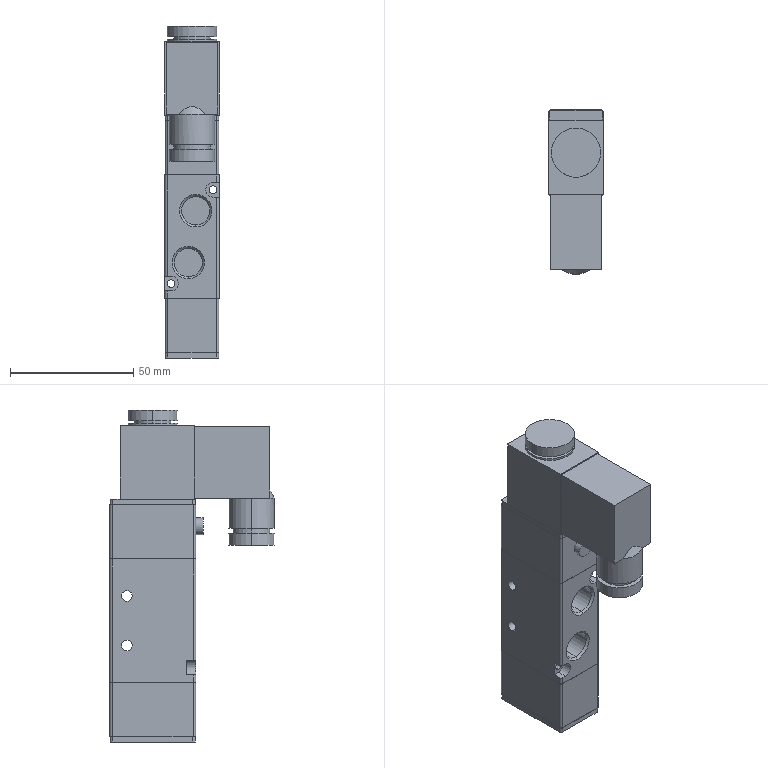Part | NX | features BREP 1 | 1 solid | 127 faces | box 22 x 66.8 x 134.6 mm | volume 113136 mm3 | cylinder 58 | plane 58 | cone 11 | commonest cylinder face diameters 2 x22 11.445 x6 3.2 x4 4.3 x4 8.566 x4 15 x4